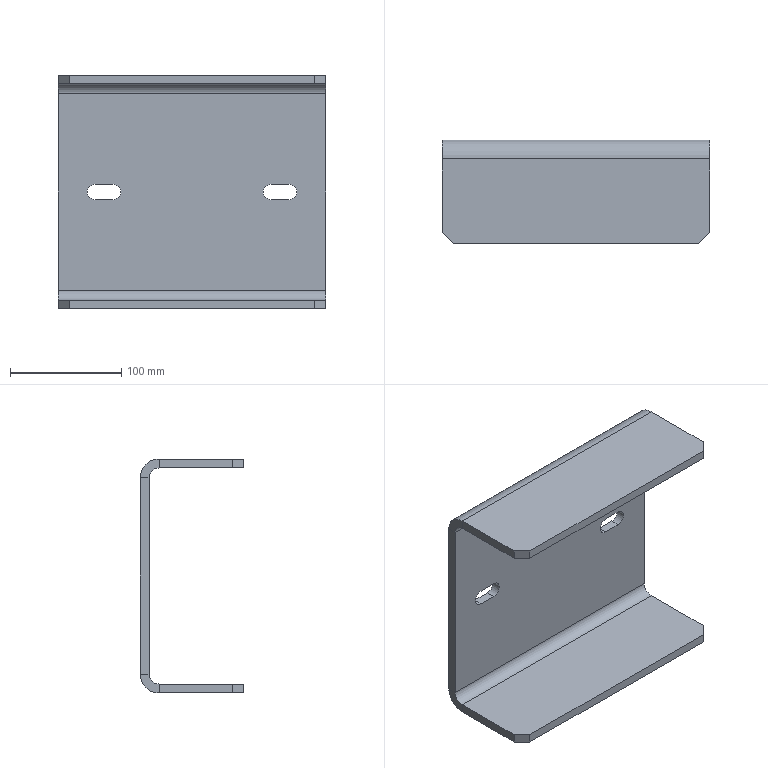Part | STEP file | _10001 | 1 solid | 34 faces | box 240 x 93 x 210 mm | volume 700527 mm3 | plane 26 | cylinder 8 | commonest cylinder face diameters 14 x4 18 x2 34 x2
STEP:
#1=CARTESIAN_POINT('',(71.,93.,235.5));
#2=VERTEX_POINT('',#1);
#3=CARTESIAN_POINT('',(71.,93.,221.5));
#4=VERTEX_POINT('',#3);
#5=CARTESIAN_POINT('',(71.,93.,228.5));
#6=DIRECTION('',(0.,-1.,0.));
#7=DIRECTION('',(0.,0.,1.));
#8=AXIS2_PLACEMENT_3D('',#5,#6,#7);
#9=CIRCLE('',#8,7.);
#10=EDGE_CURVE('',#2,#4,#9,.T.);
#11=ORIENTED_EDGE('',*,*,#10,.F.);
#12=CARTESIAN_POINT('',(71.,85.,235.5));
#13=VERTEX_POINT('',#12);
#14=CARTESIAN_POINT('',(71.,93.,235.5));
#15=DIRECTION('',(0.,-1.,0.));
#16=VECTOR('',#15,1000.);
#17=LINE('',#14,#16);
#18=EDGE_CURVE('',#2,#13,#17,.T.);
#19=ORIENTED_EDGE('',*,*,#18,.T.);
#20=CARTESIAN_POINT('',(71.,85.,221.5));
#21=VERTEX_POINT('',#20);
#22=CARTESIAN_POINT('',(71.,85.,228.5));
#23=DIRECTION('',(0.,1.,0.));
#24=DIRECTION('',(0.,0.,-1.));
#25=AXIS2_PLACEMENT_3D('',#22,#23,#24);
#26=CIRCLE('',#25,7.);
#27=EDGE_CURVE('',#21,#13,#26,.T.);
#28=ORIENTED_EDGE('',*,*,#27,.F.);
#29=CARTESIAN_POINT('',(71.,85.,221.5));
#30=DIRECTION('',(0.,1.,0.));
#31=VECTOR('',#30,1000.);
#32=LINE('',#29,#31);
#33=EDGE_CURVE('',#21,#4,#32,.T.);
#34=ORIENTED_EDGE('',*,*,#33,.T.);
#35=EDGE_LOOP('',(#11,#19,#28,#34));
#36=FACE_OUTER_BOUND('',#35,.T.);
#37=CARTESIAN_POINT('',(71.,83.,228.5));
#38=DIRECTION('',(0.,1.,0.));
#39=DIRECTION('',(0.,0.,1.));
#40=AXIS2_PLACEMENT_3D('',#37,#38,#39);
#41=CYLINDRICAL_SURFACE('',#40,7.);
#42=ADVANCED_FACE('',(#36),#41,.F.);
#43=CARTESIAN_POINT('',(87.,93.,235.5));
#44=VERTEX_POINT('',#43);
#45=CARTESIAN_POINT('',(87.,93.,235.5));
#46=DIRECTION('',(-1.,0.,0.));
#47=VECTOR('',#46,1000.);
#48=LINE('',#45,#47);
#49=EDGE_CURVE('',#44,#2,#48,.T.);
#50=ORIENTED_EDGE('',*,*,#49,.F.);
#51=CARTESIAN_POINT('',(87.,85.,235.5));
#52=VERTEX_POINT('',#51);
#53=CARTESIAN_POINT('',(87.,85.,235.5));
#54=DIRECTION('',(0.,1.,0.));
#55=VECTOR('',#54,1000.);
#56=LINE('',#53,#55);
#57=EDGE_CURVE('',#52,#44,#56,.T.);
#58=ORIENTED_EDGE('',*,*,#57,.F.);
#59=CARTESIAN_POINT('',(87.,85.,235.5));
#60=DIRECTION('',(-1.,0.,0.));
#61=VECTOR('',#60,1000.);
#62=LINE('',#59,#61);
#63=EDGE_CURVE('',#52,#13,#62,.T.);
#64=ORIENTED_EDGE('',*,*,#63,.T.);
#65=ORIENTED_EDGE('',*,*,#18,.F.);
#66=EDGE_LOOP('',(#50,#58,#64,#65));
#67=FACE_OUTER_BOUND('',#66,.T.);
#68=CARTESIAN_POINT('',(71.,83.,235.5));
#69=DIRECTION('',(0.,0.,1.));
#70=DIRECTION('',(1.,0.,0.));
#71=AXIS2_PLACEMENT_3D('',#68,#69,#70);
#72=PLANE('',#71);
#73=ADVANCED_FACE('',(#67),#72,.F.);
#74=CARTESIAN_POINT('',(87.,93.,221.5));
#75=VERTEX_POINT('',#74);
#76=CARTESIAN_POINT('',(87.,93.,228.5));
#77=DIRECTION('',(0.,-1.,0.));
#78=DIRECTION('',(0.,0.,-1.));
#79=AXIS2_PLACEMENT_3D('',#76,#77,#78);
#80=CIRCLE('',#79,7.);
#81=EDGE_CURVE('',#75,#44,#80,.T.);
#82=ORIENTED_EDGE('',*,*,#81,.F.);
#83=CARTESIAN_POINT('',(87.,85.,221.5));
#84=VERTEX_POINT('',#83);
#85=CARTESIAN_POINT('',(87.,93.,221.5));
#86=DIRECTION('',(0.,-1.,0.));
#87=VECTOR('',#86,1000.);
#88=LINE('',#85,#87);
#89=EDGE_CURVE('',#75,#84,#88,.T.);
#90=ORIENTED_EDGE('',*,*,#89,.T.);
#91=CARTESIAN_POINT('',(87.,85.,228.5));
#92=DIRECTION('',(0.,1.,0.));
#93=DIRECTION('',(0.,0.,1.));
#94=AXIS2_PLACEMENT_3D('',#91,#92,#93);
#95=CIRCLE('',#94,7.);
#96=EDGE_CURVE('',#52,#84,#95,.T.);
#97=ORIENTED_EDGE('',*,*,#96,.F.);
#98=ORIENTED_EDGE('',*,*,#57,.T.);
#99=EDGE_LOOP('',(#82,#90,#97,#98));
#100=FACE_OUTER_BOUND('',#99,.T.);
#101=CARTESIAN_POINT('',(87.,83.,228.5));
#102=DIRECTION('',(0.,1.,0.));
#103=DIRECTION('',(0.,0.,1.));
#104=AXIS2_PLACEMENT_3D('',#101,#102,#103);
#105=CYLINDRICAL_SURFACE('',#104,7.);
#106=ADVANCED_FACE('',(#100),#105,.F.);
#107=CARTESIAN_POINT('',(71.,93.,221.5));
#108=DIRECTION('',(1.,0.,0.));
#109=VECTOR('',#108,1000.);
#110=LINE('',#107,#109);
#111=EDGE_CURVE('',#4,#75,#110,.T.);
#112=ORIENTED_EDGE('',*,*,#111,.F.);
#113=ORIENTED_EDGE('',*,*,#33,.F.);
#114=CARTESIAN_POINT('',(71.,85.,221.5));
#115=DIRECTION('',(1.,0.,0.));
#116=VECTOR('',#115,1000.);
#117=LINE('',#114,#116);
#118=EDGE_CURVE('',#21,#84,#117,.T.);
#119=ORIENTED_EDGE('',*,*,#118,.T.);
#120=ORIENTED_EDGE('',*,*,#89,.F.);
#121=EDGE_LOOP('',(#112,#113,#119,#120));
#122=FACE_OUTER_BOUND('',#121,.T.);
#123=CARTESIAN_POINT('',(71.,83.,221.5));
#124=DIRECTION('',(0.,0.,-1.));
#125=DIRECTION('',(0.,-1.,0.));
#126=AXIS2_PLACEMENT_3D('',#123,#124,#125);
#127=PLANE('',#126);
#128=ADVANCED_FACE('',(#122),#127,.F.);
#129=CARTESIAN_POINT('',(-87.,93.,235.5));
#130=VERTEX_POINT('',#129);
#131=CARTESIAN_POINT('',(-87.,93.,221.5));
#132=VERTEX_POINT('',#131);
#133=CARTESIAN_POINT('',(-87.,93.,228.5));
#134=DIRECTION('',(0.,-1.,0.));
#135=DIRECTION('',(0.,0.,1.));
#136=AXIS2_PLACEMENT_3D('',#133,#134,#135);
#137=CIRCLE('',#136,7.);
#138=EDGE_CURVE('',#130,#132,#137,.T.);
#139=ORIENTED_EDGE('',*,*,#138,.F.);
#140=CARTESIAN_POINT('',(-87.,85.,235.5));
#141=VERTEX_POINT('',#140);
#142=CARTESIAN_POINT('',(-87.,93.,235.5));
#143=DIRECTION('',(0.,-1.,0.));
#144=VECTOR('',#143,1000.);
#145=LINE('',#142,#144);
#146=EDGE_CURVE('',#130,#141,#145,.T.);
#147=ORIENTED_EDGE('',*,*,#146,.T.);
#148=CARTESIAN_POINT('',(-87.,85.,221.5));
#149=VERTEX_POINT('',#148);
#150=CARTESIAN_POINT('',(-87.,85.,228.5));
#151=DIRECTION('',(0.,1.,0.));
#152=DIRECTION('',(0.,0.,-1.));
#153=AXIS2_PLACEMENT_3D('',#150,#151,#152);
#154=CIRCLE('',#153,7.);
#155=EDGE_CURVE('',#149,#141,#154,.T.);
#156=ORIENTED_EDGE('',*,*,#155,.F.);
#157=CARTESIAN_POINT('',(-87.,85.,221.5));
#158=DIRECTION('',(0.,1.,0.));
#159=VECTOR('',#158,1000.);
#160=LINE('',#157,#159);
#161=EDGE_CURVE('',#149,#132,#160,.T.);
#162=ORIENTED_EDGE('',*,*,#161,.T.);
#163=EDGE_LOOP('',(#139,#147,#156,#162));
#164=FACE_OUTER_BOUND('',#163,.T.);
#165=CARTESIAN_POINT('',(-87.,83.,228.5));
#166=DIRECTION('',(0.,1.,0.));
#167=DIRECTION('',(0.,0.,1.));
#168=AXIS2_PLACEMENT_3D('',#165,#166,#167);
#169=CYLINDRICAL_SURFACE('',#168,7.);
#170=ADVANCED_FACE('',(#164),#169,.F.);
#171=CARTESIAN_POINT('',(-71.,93.,235.5));
#172=VERTEX_POINT('',#171);
#173=CARTESIAN_POINT('',(-71.,93.,235.5));
#174=DIRECTION('',(-1.,0.,0.));
#175=VECTOR('',#174,1000.);
#176=LINE('',#173,#175);
#177=EDGE_CURVE('',#172,#130,#176,.T.);
#178=ORIENTED_EDGE('',*,*,#177,.F.);
#179=CARTESIAN_POINT('',(-71.,85.,235.5));
#180=VERTEX_POINT('',#179);
#181=CARTESIAN_POINT('',(-71.,85.,235.5));
#182=DIRECTION('',(0.,1.,0.));
#183=VECTOR('',#182,1000.);
#184=LINE('',#181,#183);
#185=EDGE_CURVE('',#180,#172,#184,.T.);
#186=ORIENTED_EDGE('',*,*,#185,.F.);
#187=CARTESIAN_POINT('',(-71.,85.,235.5));
#188=DIRECTION('',(-1.,0.,0.));
#189=VECTOR('',#188,1000.);
#190=LINE('',#187,#189);
#191=EDGE_CURVE('',#180,#141,#190,.T.);
#192=ORIENTED_EDGE('',*,*,#191,.T.);
#193=ORIENTED_EDGE('',*,*,#146,.F.);
#194=EDGE_LOOP('',(#178,#186,#192,#193));
#195=FACE_OUTER_BOUND('',#194,.T.);
#196=CARTESIAN_POINT('',(-87.,83.,235.5));
#197=DIRECTION('',(0.,0.,1.));
#198=DIRECTION('',(1.,0.,0.));
#199=AXIS2_PLACEMENT_3D('',#196,#197,#198);
#200=PLANE('',#199);
#201=ADVANCED_FACE('',(#195),#200,.F.);
#202=CARTESIAN_POINT('',(-71.,93.,221.5));
#203=VERTEX_POINT('',#202);
#204=CARTESIAN_POINT('',(-71.,93.,228.5));
#205=DIRECTION('',(0.,-1.,0.));
#206=DIRECTION('',(0.,0.,-1.));
#207=AXIS2_PLACEMENT_3D('',#204,#205,#206);
#208=CIRCLE('',#207,7.);
#209=EDGE_CURVE('',#203,#172,#208,.T.);
#210=ORIENTED_EDGE('',*,*,#209,.F.);
#211=CARTESIAN_POINT('',(-71.,85.,221.5));
#212=VERTEX_POINT('',#211);
#213=CARTESIAN_POINT('',(-71.,93.,221.5));
#214=DIRECTION('',(0.,-1.,0.));
#215=VECTOR('',#214,1000.);
#216=LINE('',#213,#215);
#217=EDGE_CURVE('',#203,#212,#216,.T.);
#218=ORIENTED_EDGE('',*,*,#217,.T.);
#219=CARTESIAN_POINT('',(-71.,85.,228.5));
#220=DIRECTION('',(0.,1.,0.));
#221=DIRECTION('',(0.,0.,1.));
#222=AXIS2_PLACEMENT_3D('',#219,#220,#221);
#223=CIRCLE('',#222,7.);
#224=EDGE_CURVE('',#180,#212,#223,.T.);
#225=ORIENTED_EDGE('',*,*,#224,.F.);
#226=ORIENTED_EDGE('',*,*,#185,.T.);
#227=EDGE_LOOP('',(#210,#218,#225,#226));
#228=FACE_OUTER_BOUND('',#227,.T.);
#229=CARTESIAN_POINT('',(-71.,83.,228.5));
#230=DIRECTION('',(0.,1.,0.));
#231=DIRECTION('',(0.,0.,1.));
#232=AXIS2_PLACEMENT_3D('',#229,#230,#231);
#233=CYLINDRICAL_SURFACE('',#232,7.);
#234=ADVANCED_FACE('',(#228),#233,.F.);
#235=CARTESIAN_POINT('',(-87.,93.,221.5));
#236=DIRECTION('',(1.,0.,0.));
#237=VECTOR('',#236,1000.);
#238=LINE('',#235,#237);
#239=EDGE_CURVE('',#132,#203,#238,.T.);
#240=ORIENTED_EDGE('',*,*,#239,.F.);
#241=ORIENTED_EDGE('',*,*,#161,.F.);
#242=CARTESIAN_POINT('',(-87.,85.,221.5));
#243=DIRECTION('',(1.,0.,0.));
#244=VECTOR('',#243,1000.);
#245=LINE('',#242,#244);
#246=EDGE_CURVE('',#149,#212,#245,.T.);
#247=ORIENTED_EDGE('',*,*,#246,.T.);
#248=ORIENTED_EDGE('',*,*,#217,.F.);
#249=EDGE_LOOP('',(#240,#241,#247,#248));
#250=FACE_OUTER_BOUND('',#249,.T.);
#251=CARTESIAN_POINT('',(-87.,83.,221.5));
#252=DIRECTION('',(0.,0.,-1.));
#253=DIRECTION('',(0.,-1.,0.));
#254=AXIS2_PLACEMENT_3D('',#251,#252,#253);
#255=PLANE('',#254);
#256=ADVANCED_FACE('',(#250),#255,.F.);
#257=CARTESIAN_POINT('',(-110.,0.,325.5));
#258=VERTEX_POINT('',#257);
#259=CARTESIAN_POINT('',(-110.,0.,333.5));
#260=VERTEX_POINT('',#259);
#261=CARTESIAN_POINT('',(-110.,0.,325.5));
#262=DIRECTION('',(0.,0.,1.));
#263=VECTOR('',#262,1000.);
#264=LINE('',#261,#263);
#265=EDGE_CURVE('',#258,#260,#264,.T.);
#266=ORIENTED_EDGE('',*,*,#265,.T.);
#267=CARTESIAN_POINT('',(-120.,10.,333.5));
#268=VERTEX_POINT('',#267);
#269=CARTESIAN_POINT('',(-120.,10.,333.5));
#270=DIRECTION('',(0.7071,-0.7071,0.));
#271=VECTOR('',#270,1000.);
#272=LINE('',#269,#271);
#273=EDGE_CURVE('',#268,#260,#272,.T.);
#274=ORIENTED_EDGE('',*,*,#273,.F.);
#275=CARTESIAN_POINT('',(-120.,10.,325.5));
#276=VERTEX_POINT('',#275);
#277=CARTESIAN_POINT('',(-120.,10.,333.5));
#278=DIRECTION('',(0.,0.,-1.));
#279=VECTOR('',#278,1000.);
#280=LINE('',#277,#279);
#281=EDGE_CURVE('',#268,#276,#280,.T.);
#282=ORIENTED_EDGE('',*,*,#281,.T.);
#283=CARTESIAN_POINT('',(-110.,0.,325.5));
#284=DIRECTION('',(-0.7071,0.7071,0.));
#285=VECTOR('',#284,1000.);
#286=LINE('',#283,#285);
#287=EDGE_CURVE('',#258,#276,#286,.T.);
#288=ORIENTED_EDGE('',*,*,#287,.F.);
#289=EDGE_LOOP('',(#266,#274,#282,#288));
#290=FACE_OUTER_BOUND('',#289,.T.);
#291=CARTESIAN_POINT('',(-120.,10.,316.5));
#292=DIRECTION('',(0.7071,0.7071,0.));
#293=DIRECTION('',(0.,0.,-1.));
#294=AXIS2_PLACEMENT_3D('',#291,#292,#293);
#295=PLANE('',#294);
#296=ADVANCED_FACE('',(#290),#295,.F.);
#297=CARTESIAN_POINT('',(120.,10.,325.5));
#298=VERTEX_POINT('',#297);
#299=CARTESIAN_POINT('',(120.,10.,333.5));
#300=VERTEX_POINT('',#299);
#301=CARTESIAN_POINT('',(120.,10.,325.5));
#302=DIRECTION('',(0.,0.,1.));
#303=VECTOR('',#302,1000.);
#304=LINE('',#301,#303);
#305=EDGE_CURVE('',#298,#300,#304,.T.);
#306=ORIENTED_EDGE('',*,*,#305,.T.);
#307=CARTESIAN_POINT('',(110.,0.,333.5));
#308=VERTEX_POINT('',#307);
#309=CARTESIAN_POINT('',(110.,0.,333.5));
#310=DIRECTION('',(0.7071,0.7071,0.));
#311=VECTOR('',#310,1000.);
#312=LINE('',#309,#311);
#313=EDGE_CURVE('',#308,#300,#312,.T.);
#314=ORIENTED_EDGE('',*,*,#313,.F.);
#315=CARTESIAN_POINT('',(110.,0.,325.5));
#316=VERTEX_POINT('',#315);
#317=CARTESIAN_POINT('',(110.,0.,333.5));
#318=DIRECTION('',(0.,0.,-1.));
#319=VECTOR('',#318,1000.);
#320=LINE('',#317,#319);
#321=EDGE_CURVE('',#308,#316,#320,.T.);
#322=ORIENTED_EDGE('',*,*,#321,.T.);
#323=CARTESIAN_POINT('',(120.,10.,325.5));
#324=DIRECTION('',(-0.7071,-0.7071,0.));
#325=VECTOR('',#324,1000.);
#326=LINE('',#323,#325);
#327=EDGE_CURVE('',#298,#316,#326,.T.);
#328=ORIENTED_EDGE('',*,*,#327,.F.);
#329=EDGE_LOOP('',(#306,#314,#322,#328));
#330=FACE_OUTER_BOUND('',#329,.T.);
#331=CARTESIAN_POINT('',(110.,0.,325.5));
#332=DIRECTION('',(-0.7071,0.7071,0.));
#333=DIRECTION('',(0.,0.,1.));
#334=AXIS2_PLACEMENT_3D('',#331,#332,#333);
#335=PLANE('',#334);
#336=ADVANCED_FACE('',(#330),#335,.F.);
#337=ORIENTED_EDGE('',*,*,#305,.F.);
#338=CARTESIAN_POINT('',(120.,76.,325.5));
#339=VERTEX_POINT('',#338);
#340=CARTESIAN_POINT('',(120.,76.,325.5));
#341=DIRECTION('',(0.,-1.,0.));
#342=VECTOR('',#341,1000.);
#343=LINE('',#340,#342);
#344=EDGE_CURVE('',#339,#298,#343,.T.);
#345=ORIENTED_EDGE('',*,*,#344,.F.);
#346=CARTESIAN_POINT('',(120.,76.,333.5));
#347=VERTEX_POINT('',#346);
#348=CARTESIAN_POINT('',(120.,76.,333.5));
#349=DIRECTION('',(0.,0.,-1.));
#350=VECTOR('',#349,1000.);
#351=LINE('',#348,#350);
#352=EDGE_CURVE('',#347,#339,#351,.T.);
#353=ORIENTED_EDGE('',*,*,#352,.F.);
#354=CARTESIAN_POINT('',(120.,76.,333.5));
#355=DIRECTION('',(0.,-1.,0.));
#356=VECTOR('',#355,1000.);
#357=LINE('',#354,#356);
#358=EDGE_CURVE('',#347,#300,#357,.T.);
#359=ORIENTED_EDGE('',*,*,#358,.T.);
#360=EDGE_LOOP('',(#337,#345,#353,#359));
#361=FACE_OUTER_BOUND('',#360,.T.);
#362=CARTESIAN_POINT('',(120.,76.,140.5));
#363=DIRECTION('',(1.,0.,0.));
#364=DIRECTION('',(0.,1.,0.));
#365=AXIS2_PLACEMENT_3D('',#362,#363,#364);
#366=PLANE('',#365);
#367=ADVANCED_FACE('',(#361),#366,.T.);
#368=CARTESIAN_POINT('',(120.,93.,316.5));
#369=VERTEX_POINT('',#368);
#370=CARTESIAN_POINT('',(120.,76.,316.5));
#371=DIRECTION('',(1.,0.,0.));
#372=DIRECTION('',(0.,1.,0.));
#373=AXIS2_PLACEMENT_3D('',#370,#371,#372);
#374=CIRCLE('',#373,17.);
#375=EDGE_CURVE('',#369,#347,#374,.T.);
#376=ORIENTED_EDGE('',*,*,#375,.T.);
#377=ORIENTED_EDGE('',*,*,#352,.T.);
#378=CARTESIAN_POINT('',(120.,85.,316.5));
#379=VERTEX_POINT('',#378);
#380=CARTESIAN_POINT('',(120.,76.,316.5));
#381=DIRECTION('',(-1.,0.,0.));
#382=DIRECTION('',(0.,0.,1.));
#383=AXIS2_PLACEMENT_3D('',#380,#381,#382);
#384=CIRCLE('',#383,9.);
#385=EDGE_CURVE('',#339,#379,#384,.T.);
#386=ORIENTED_EDGE('',*,*,#385,.T.);
#387=CARTESIAN_POINT('',(120.,85.,316.5));
#388=DIRECTION('',(0.,1.,0.));
#389=VECTOR('',#388,1000.);
#390=LINE('',#387,#389);
#391=EDGE_CURVE('',#379,#369,#390,.T.);
#392=ORIENTED_EDGE('',*,*,#391,.T.);
#393=EDGE_LOOP('',(#376,#377,#386,#392));
#394=FACE_OUTER_BOUND('',#393,.T.);
#395=CARTESIAN_POINT('',(120.,93.,316.5));
#396=DIRECTION('',(1.,0.,0.));
#397=DIRECTION('',(0.,1.,0.));
#398=AXIS2_PLACEMENT_3D('',#395,#396,#397);
#399=PLANE('',#398);
#400=ADVANCED_FACE('',(#394),#399,.T.);
#401=CARTESIAN_POINT('',(-120.,76.,333.5));
#402=VERTEX_POINT('',#401);
#403=CARTESIAN_POINT('',(-120.,76.,333.5));
#404=DIRECTION('',(1.,0.,0.));
#405=VECTOR('',#404,1000.);
#406=LINE('',#403,#405);
#407=EDGE_CURVE('',#402,#347,#406,.T.);
#408=ORIENTED_EDGE('',*,*,#407,.T.);
#409=ORIENTED_EDGE('',*,*,#375,.F.);
#410=CARTESIAN_POINT('',(-120.,93.,316.5));
#411=VERTEX_POINT('',#410);
#412=CARTESIAN_POINT('',(120.,93.,316.5));
#413=DIRECTION('',(-1.,0.,0.));
#414=VECTOR('',#413,1000.);
#415=LINE('',#412,#414);
#416=EDGE_CURVE('',#369,#411,#415,.T.);
#417=ORIENTED_EDGE('',*,*,#416,.T.);
#418=CARTESIAN_POINT('',(-120.,76.,316.5));
#419=DIRECTION('',(-1.,0.,0.));
#420=DIRECTION('',(0.,0.,1.));
#421=AXIS2_PLACEMENT_3D('',#418,#419,#420);
#422=CIRCLE('',#421,17.);
#423=EDGE_CURVE('',#402,#411,#422,.T.);
#424=ORIENTED_EDGE('',*,*,#423,.F.);
#425=EDGE_LOOP('',(#408,#409,#417,#424));
#426=FACE_OUTER_BOUND('',#425,.T.);
#427=CARTESIAN_POINT('',(120.,76.,316.5));
#428=DIRECTION('',(-1.,0.,0.));
#429=DIRECTION('',(0.,0.,1.));
#430=AXIS2_PLACEMENT_3D('',#427,#428,#429);
#431=CYLINDRICAL_SURFACE('',#430,17.);
#432=ADVANCED_FACE('',(#426),#431,.T.);
#433=ORIENTED_EDGE('',*,*,#273,.T.);
#434=CARTESIAN_POINT('',(-110.,0.,333.5));
#435=DIRECTION('',(1.,0.,0.));
#436=VECTOR('',#435,1000.);
#437=LINE('',#434,#436);
#438=EDGE_CURVE('',#260,#308,#437,.T.);
#439=ORIENTED_EDGE('',*,*,#438,.T.);
#440=ORIENTED_EDGE('',*,*,#313,.T.);
#441=ORIENTED_EDGE('',*,*,#358,.F.);
#442=ORIENTED_EDGE('',*,*,#407,.F.);
#443=CARTESIAN_POINT('',(-120.,76.,333.5));
#444=DIRECTION('',(0.,-1.,0.));
#445=VECTOR('',#444,1000.);
#446=LINE('',#443,#445);
#447=EDGE_CURVE('',#402,#268,#446,.T.);
#448=ORIENTED_EDGE('',*,*,#447,.T.);
#449=EDGE_LOOP('',(#433,#439,#440,#441,#442,#448));
#450=FACE_OUTER_BOUND('',#449,.T.);
#451=CARTESIAN_POINT('',(120.,0.,333.5));
#452=DIRECTION('',(0.,0.,1.));
#453=DIRECTION('',(1.,0.,0.));
#454=AXIS2_PLACEMENT_3D('',#451,#452,#453);
#455=PLANE('',#454);
#456=ADVANCED_FACE('',(#450),#455,.T.);
#457=ORIENTED_EDGE('',*,*,#265,.F.);
#458=CARTESIAN_POINT('',(-110.,0.,325.5));
#459=DIRECTION('',(1.,0.,0.));
#460=VECTOR('',#459,1000.);
#461=LINE('',#458,#460);
#462=EDGE_CURVE('',#258,#316,#461,.T.);
#463=ORIENTED_EDGE('',*,*,#462,.T.);
#464=ORIENTED_EDGE('',*,*,#321,.F.);
#465=ORIENTED_EDGE('',*,*,#438,.F.);
#466=EDGE_LOOP('',(#457,#463,#464,#465));
#467=FACE_OUTER_BOUND('',#466,.T.);
#468=CARTESIAN_POINT('',(120.,0.,325.5));
#469=DIRECTION('',(0.,-1.,0.));
#470=DIRECTION('',(0.,0.,-1.));
#471=AXIS2_PLACEMENT_3D('',#468,#469,#470);
#472=PLANE('',#471);
#473=ADVANCED_FACE('',(#467),#472,.T.);
#474=ORIENTED_EDGE('',*,*,#287,.T.);
#475=CARTESIAN_POINT('',(-120.,76.,325.5));
#476=VERTEX_POINT('',#475);
#477=CARTESIAN_POINT('',(-120.,76.,325.5));
#478=DIRECTION('',(0.,-1.,0.));
#479=VECTOR('',#478,1000.);
#480=LINE('',#477,#479);
#481=EDGE_CURVE('',#476,#276,#480,.T.);
#482=ORIENTED_EDGE('',*,*,#481,.F.);
#483=CARTESIAN_POINT('',(120.,76.,325.5));
#484=DIRECTION('',(-1.,0.,0.));
#485=VECTOR('',#484,1000.);
#486=LINE('',#483,#485);
#487=EDGE_CURVE('',#339,#476,#486,.T.);
#488=ORIENTED_EDGE('',*,*,#487,.F.);
#489=ORIENTED_EDGE('',*,*,#344,.T.);
#490=ORIENTED_EDGE('',*,*,#327,.T.);
#491=ORIENTED_EDGE('',*,*,#462,.F.);
#492=EDGE_LOOP('',(#474,#482,#488,#489,#490,#491));
#493=FACE_OUTER_BOUND('',#492,.T.);
#494=CARTESIAN_POINT('',(120.,0.,325.5));
#495=DIRECTION('',(0.,0.,1.));
#496=DIRECTION('',(1.,0.,0.));
#497=AXIS2_PLACEMENT_3D('',#494,#495,#496);
#498=PLANE('',#497);
#499=ADVANCED_FACE('',(#493),#498,.F.);
#500=ORIENTED_EDGE('',*,*,#281,.F.);
#501=ORIENTED_EDGE('',*,*,#447,.F.);
#502=CARTESIAN_POINT('',(-120.,76.,325.5));
#503=DIRECTION('',(0.,0.,1.));
#504=VECTOR('',#503,1000.);
#505=LINE('',#502,#504);
#506=EDGE_CURVE('',#476,#402,#505,.T.);
#507=ORIENTED_EDGE('',*,*,#506,.F.);
#508=ORIENTED_EDGE('',*,*,#481,.T.);
#509=EDGE_LOOP('',(#500,#501,#507,#508));
#510=FACE_OUTER_BOUND('',#509,.T.);
#511=CARTESIAN_POINT('',(-120.,85.,316.5));
#512=DIRECTION('',(-1.,0.,0.));
#513=DIRECTION('',(0.,0.,1.));
#514=AXIS2_PLACEMENT_3D('',#511,#512,#513);
#515=PLANE('',#514);
#516=ADVANCED_FACE('',(#510),#515,.T.);
#517=ORIENTED_EDGE('',*,*,#423,.T.);
#518=CARTESIAN_POINT('',(-120.,85.,316.5));
#519=VERTEX_POINT('',#518);
#520=CARTESIAN_POINT('',(-120.,93.,316.5));
#521=DIRECTION('',(0.,-1.,0.));
#522=VECTOR('',#521,1000.);
#523=LINE('',#520,#522);
#524=EDGE_CURVE('',#411,#519,#523,.T.);
#525=ORIENTED_EDGE('',*,*,#524,.T.);
#526=CARTESIAN_POINT('',(-120.,76.,316.5));
#527=DIRECTION('',(1.,0.,0.));
#528=DIRECTION('',(0.,1.,0.));
#529=AXIS2_PLACEMENT_3D('',#526,#527,#528);
#530=CIRCLE('',#529,9.);
#531=EDGE_CURVE('',#519,#476,#530,.T.);
#532=ORIENTED_EDGE('',*,*,#531,.T.);
#533=ORIENTED_EDGE('',*,*,#506,.T.);
#534=EDGE_LOOP('',(#517,#525,#532,#533));
#535=FACE_OUTER_BOUND('',#534,.T.);
#536=CARTESIAN_POINT('',(-120.,76.,333.5));
#537=DIRECTION('',(-1.,0.,0.));
#538=DIRECTION('',(0.,0.,1.));
#539=AXIS2_PLACEMENT_3D('',#536,#537,#538);
#540=PLANE('',#539);
#541=ADVANCED_FACE('',(#535),#540,.T.);
#542=CARTESIAN_POINT('',(-120.,85.,316.5));
#543=DIRECTION('',(1.,0.,0.));
#544=VECTOR('',#543,1000.);
#545=LINE('',#542,#544);
#546=EDGE_CURVE('',#519,#379,#545,.T.);
#547=ORIENTED_EDGE('',*,*,#546,.T.);
#548=ORIENTED_EDGE('',*,*,#385,.F.);
#549=ORIENTED_EDGE('',*,*,#487,.T.);
#550=ORIENTED_EDGE('',*,*,#531,.F.);
#551=EDGE_LOOP('',(#547,#548,#549,#550));
#552=FACE_OUTER_BOUND('',#551,.T.);
#553=CARTESIAN_POINT('',(120.,76.,316.5));
#554=DIRECTION('',(-1.,0.,0.));
#555=DIRECTION('',(0.,0.,1.));
#556=AXIS2_PLACEMENT_3D('',#553,#554,#555);
#557=CYLINDRICAL_SURFACE('',#556,9.);
#558=ADVANCED_FACE('',(#552),#557,.F.);
#559=ORIENTED_EDGE('',*,*,#27,.T.);
#560=ORIENTED_EDGE('',*,*,#63,.F.);
#561=ORIENTED_EDGE('',*,*,#96,.T.);
#562=ORIENTED_EDGE('',*,*,#118,.F.);
#563=EDGE_LOOP('',(#559,#560,#561,#562));
#564=FACE_BOUND('',#563,.T.);
#565=ORIENTED_EDGE('',*,*,#155,.T.);
#566=ORIENTED_EDGE('',*,*,#191,.F.);
#567=ORIENTED_EDGE('',*,*,#224,.T.);
#568=ORIENTED_EDGE('',*,*,#246,.F.);
#569=EDGE_LOOP('',(#565,#566,#567,#568));
#570=FACE_BOUND('',#569,.T.);
#571=CARTESIAN_POINT('',(120.,85.,140.5));
#572=VERTEX_POINT('',#571);
#573=CARTESIAN_POINT('',(-120.,85.,140.5));
#574=VERTEX_POINT('',#573);
#575=CARTESIAN_POINT('',(120.,85.,140.5));
#576=DIRECTION('',(-1.,0.,0.));
#577=VECTOR('',#576,1000.);
#578=LINE('',#575,#577);
#579=EDGE_CURVE('',#572,#574,#578,.T.);
#580=ORIENTED_EDGE('',*,*,#579,.F.);
#581=CARTESIAN_POINT('',(120.,85.,140.5));
#582=DIRECTION('',(0.,0.,1.));
#583=VECTOR('',#582,1000.);
#584=LINE('',#581,#583);
#585=EDGE_CURVE('',#572,#379,#584,.T.);
#586=ORIENTED_EDGE('',*,*,#585,.T.);
#587=ORIENTED_EDGE('',*,*,#546,.F.);
#588=CARTESIAN_POINT('',(-120.,85.,140.5));
#589=DIRECTION('',(0.,0.,1.));
#590=VECTOR('',#589,1000.);
#591=LINE('',#588,#590);
#592=EDGE_CURVE('',#574,#519,#591,.T.);
#593=ORIENTED_EDGE('',*,*,#592,.F.);
#594=EDGE_LOOP('',(#580,#586,#587,#593));
#595=FACE_OUTER_BOUND('',#594,.T.);
#596=CARTESIAN_POINT('',(120.,85.,333.5));
#597=DIRECTION('',(0.,1.,0.));
#598=DIRECTION('',(1.,0.,0.));
#599=AXIS2_PLACEMENT_3D('',#596,#597,#598);
#600=PLANE('',#599);
#601=ADVANCED_FACE('',(#564,#570,#595),#600,.F.);
#602=CARTESIAN_POINT('',(-120.,76.,131.5));
#603=VERTEX_POINT('',#602);
#604=CARTESIAN_POINT('',(120.,76.,131.5));
#605=VERTEX_POINT('',#604);
#606=CARTESIAN_POINT('',(-120.,76.,131.5));
#607=DIRECTION('',(1.,0.,0.));
#608=VECTOR('',#607,1000.);
#609=LINE('',#606,#608);
#610=EDGE_CURVE('',#603,#605,#609,.T.);
#611=ORIENTED_EDGE('',*,*,#610,.T.);
#612=CARTESIAN_POINT('',(120.,76.,140.5));
#613=DIRECTION('',(-1.,0.,0.));
#614=DIRECTION('',(0.,1.,0.));
#615=AXIS2_PLACEMENT_3D('',#612,#613,#614);
#616=CIRCLE('',#615,9.);
#617=EDGE_CURVE('',#572,#605,#616,.T.);
#618=ORIENTED_EDGE('',*,*,#617,.F.);
#619=ORIENTED_EDGE('',*,*,#579,.T.);
#620=CARTESIAN_POINT('',(-120.,76.,140.5));
#621=DIRECTION('',(1.,0.,0.));
#622=DIRECTION('',(0.,0.,-1.));
#623=AXIS2_PLACEMENT_3D('',#620,#621,#622);
#624=CIRCLE('',#623,9.);
#625=EDGE_CURVE('',#603,#574,#624,.T.);
#626=ORIENTED_EDGE('',*,*,#625,.F.);
#627=EDGE_LOOP('',(#611,#618,#619,#626));
#628=FACE_OUTER_BOUND('',#627,.T.);
#629=CARTESIAN_POINT('',(120.,76.,140.5));
#630=DIRECTION('',(-1.,0.,0.));
#631=DIRECTION('',(0.,0.,1.));
#632=AXIS2_PLACEMENT_3D('',#629,#630,#631);
#633=CYLINDRICAL_SURFACE('',#632,9.);
#634=ADVANCED_FACE('',(#628),#633,.F.);
#635=CARTESIAN_POINT('',(-110.,0.,123.5));
#636=VERTEX_POINT('',#635);
#637=CARTESIAN_POINT('',(-110.,0.,131.5));
#638=VERTEX_POINT('',#637);
#639=CARTESIAN_POINT('',(-110.,0.,123.5));
#640=DIRECTION('',(0.,0.,1.));
#641=VECTOR('',#640,1000.);
#642=LINE('',#639,#641);
#643=EDGE_CURVE('',#636,#638,#642,.T.);
#644=ORIENTED_EDGE('',*,*,#643,.T.);
#645=CARTESIAN_POINT('',(-120.,10.,131.5));
#646=VERTEX_POINT('',#645);
#647=CARTESIAN_POINT('',(-120.,10.,131.5));
#648=DIRECTION('',(0.7071,-0.7071,0.));
#649=VECTOR('',#648,1000.);
#650=LINE('',#647,#649);
#651=EDGE_CURVE('',#646,#638,#650,.T.);
#652=ORIENTED_EDGE('',*,*,#651,.F.);
#653=CARTESIAN_POINT('',(-120.,10.,123.5));
#654=VERTEX_POINT('',#653);
#655=CARTESIAN_POINT('',(-120.,10.,131.5));
#656=DIRECTION('',(0.,0.,-1.));
#657=VECTOR('',#656,1000.);
#658=LINE('',#655,#657);
#659=EDGE_CURVE('',#646,#654,#658,.T.);
#660=ORIENTED_EDGE('',*,*,#659,.T.);
#661=CARTESIAN_POINT('',(-110.,0.,123.5));
#662=DIRECTION('',(-0.7071,0.7071,0.));
#663=VECTOR('',#662,1000.);
#664=LINE('',#661,#663);
#665=EDGE_CURVE('',#636,#654,#664,.T.);
#666=ORIENTED_EDGE('',*,*,#665,.F.);
#667=EDGE_LOOP('',(#644,#652,#660,#666));
#668=FACE_OUTER_BOUND('',#667,.T.);
#669=CARTESIAN_POINT('',(-120.,10.,140.5));
#670=DIRECTION('',(-0.7071,-0.7071,0.));
#671=DIRECTION('',(-0.7071,0.7071,0.));
#672=AXIS2_PLACEMENT_3D('',#669,#670,#671);
#673=PLANE('',#672);
#674=ADVANCED_FACE('',(#668),#673,.T.);
#675=CARTESIAN_POINT('',(120.,10.,123.5));
#676=VERTEX_POINT('',#675);
#677=CARTESIAN_POINT('',(120.,10.,131.5));
#678=VERTEX_POINT('',#677);
#679=CARTESIAN_POINT('',(120.,10.,123.5));
#680=DIRECTION('',(0.,0.,1.));
#681=VECTOR('',#680,1000.);
#682=LINE('',#679,#681);
#683=EDGE_CURVE('',#676,#678,#682,.T.);
#684=ORIENTED_EDGE('',*,*,#683,.T.);
#685=CARTESIAN_POINT('',(110.,0.,131.5));
#686=VERTEX_POINT('',#685);
#687=CARTESIAN_POINT('',(110.,0.,131.5));
#688=DIRECTION('',(0.7071,0.7071,0.));
#689=VECTOR('',#688,1000.);
#690=LINE('',#687,#689);
#691=EDGE_CURVE('',#686,#678,#690,.T.);
#692=ORIENTED_EDGE('',*,*,#691,.F.);
#693=CARTESIAN_POINT('',(110.,0.,123.5));
#694=VERTEX_POINT('',#693);
#695=CARTESIAN_POINT('',(110.,0.,131.5));
#696=DIRECTION('',(0.,0.,-1.));
#697=VECTOR('',#696,1000.);
#698=LINE('',#695,#697);
#699=EDGE_CURVE('',#686,#694,#698,.T.);
#700=ORIENTED_EDGE('',*,*,#699,.T.);
#701=CARTESIAN_POINT('',(120.,10.,123.5));
#702=DIRECTION('',(-0.7071,-0.7071,0.));
#703=VECTOR('',#702,1000.);
#704=LINE('',#701,#703);
#705=EDGE_CURVE('',#676,#694,#704,.T.);
#706=ORIENTED_EDGE('',*,*,#705,.F.);
#707=EDGE_LOOP('',(#684,#692,#700,#706));
#708=FACE_OUTER_BOUND('',#707,.T.);
#709=CARTESIAN_POINT('',(110.,0.,123.5));
#710=DIRECTION('',(-0.7071,0.7071,0.));
#711=DIRECTION('',(0.,0.,1.));
#712=AXIS2_PLACEMENT_3D('',#709,#710,#711);
#713=PLANE('',#712);
#714=ADVANCED_FACE('',(#708),#713,.F.);
#715=ORIENTED_EDGE('',*,*,#643,.F.);
#716=CARTESIAN_POINT('',(-110.,0.,123.5));
#717=DIRECTION('',(1.,0.,0.));
#718=VECTOR('',#717,1000.);
#719=LINE('',#716,#718);
#720=EDGE_CURVE('',#636,#694,#719,.T.);
#721=ORIENTED_EDGE('',*,*,#720,.T.);
#722=ORIENTED_EDGE('',*,*,#699,.F.);
#723=CARTESIAN_POINT('',(-110.,0.,131.5));
#724=DIRECTION('',(1.,0.,0.));
#725=VECTOR('',#724,1000.);
#726=LINE('',#723,#725);
#727=EDGE_CURVE('',#638,#686,#726,.T.);
#728=ORIENTED_EDGE('',*,*,#727,.F.);
#729=EDGE_LOOP('',(#715,#721,#722,#728));
#730=FACE_OUTER_BOUND('',#729,.T.);
#731=CARTESIAN_POINT('',(120.,0.,123.5));
#732=DIRECTION('',(0.,-1.,0.));
#733=DIRECTION('',(0.,0.,-1.));
#734=AXIS2_PLACEMENT_3D('',#731,#732,#733);
#735=PLANE('',#734);
#736=ADVANCED_FACE('',(#730),#735,.T.);
#737=ORIENTED_EDGE('',*,*,#665,.T.);
#738=CARTESIAN_POINT('',(-120.,76.,123.5));
#739=VERTEX_POINT('',#738);
#740=CARTESIAN_POINT('',(-120.,10.,123.5));
#741=DIRECTION('',(0.,1.,0.));
#742=VECTOR('',#741,1000.);
#743=LINE('',#740,#742);
#744=EDGE_CURVE('',#654,#739,#743,.T.);
#745=ORIENTED_EDGE('',*,*,#744,.T.);
#746=CARTESIAN_POINT('',(120.,76.,123.5));
#747=VERTEX_POINT('',#746);
#748=CARTESIAN_POINT('',(120.,76.,123.5));
#749=DIRECTION('',(-1.,0.,0.));
#750=VECTOR('',#749,1000.);
#751=LINE('',#748,#750);
#752=EDGE_CURVE('',#747,#739,#751,.T.);
#753=ORIENTED_EDGE('',*,*,#752,.F.);
#754=CARTESIAN_POINT('',(120.,10.,123.5));
#755=DIRECTION('',(0.,1.,0.));
#756=VECTOR('',#755,1000.);
#757=LINE('',#754,#756);
#758=EDGE_CURVE('',#676,#747,#757,.T.);
#759=ORIENTED_EDGE('',*,*,#758,.F.);
#760=ORIENTED_EDGE('',*,*,#705,.T.);
#761=ORIENTED_EDGE('',*,*,#720,.F.);
#762=EDGE_LOOP('',(#737,#745,#753,#759,#760,#761));
#763=FACE_OUTER_BOUND('',#762,.T.);
#764=CARTESIAN_POINT('',(120.,93.,123.5));
#765=DIRECTION('',(0.,0.,-1.));
#766=DIRECTION('',(0.,-1.,0.));
#767=AXIS2_PLACEMENT_3D('',#764,#765,#766);
#768=PLANE('',#767);
#769=ADVANCED_FACE('',(#763),#768,.T.);
#770=ORIENTED_EDGE('',*,*,#659,.F.);
#771=CARTESIAN_POINT('',(-120.,10.,131.5));
#772=DIRECTION('',(0.,1.,0.));
#773=VECTOR('',#772,1000.);
#774=LINE('',#771,#773);
#775=EDGE_CURVE('',#646,#603,#774,.T.);
#776=ORIENTED_EDGE('',*,*,#775,.T.);
#777=CARTESIAN_POINT('',(-120.,76.,123.5));
#778=DIRECTION('',(0.,0.,1.));
#779=VECTOR('',#778,1000.);
#780=LINE('',#777,#779);
#781=EDGE_CURVE('',#739,#603,#780,.T.);
#782=ORIENTED_EDGE('',*,*,#781,.F.);
#783=ORIENTED_EDGE('',*,*,#744,.F.);
#784=EDGE_LOOP('',(#770,#776,#782,#783));
#785=FACE_OUTER_BOUND('',#784,.T.);
#786=CARTESIAN_POINT('',(-120.,76.,140.5));
#787=DIRECTION('',(1.,0.,0.));
#788=DIRECTION('',(0.,1.,0.));
#789=AXIS2_PLACEMENT_3D('',#786,#787,#788);
#790=PLANE('',#789);
#791=ADVANCED_FACE('',(#785),#790,.F.);
#792=ORIENTED_EDGE('',*,*,#651,.T.);
#793=ORIENTED_EDGE('',*,*,#727,.T.);
#794=ORIENTED_EDGE('',*,*,#691,.T.);
#795=CARTESIAN_POINT('',(120.,10.,131.5));
#796=DIRECTION('',(0.,1.,0.));
#797=VECTOR('',#796,1000.);
#798=LINE('',#795,#797);
#799=EDGE_CURVE('',#678,#605,#798,.T.);
#800=ORIENTED_EDGE('',*,*,#799,.T.);
#801=ORIENTED_EDGE('',*,*,#610,.F.);
#802=ORIENTED_EDGE('',*,*,#775,.F.);
#803=EDGE_LOOP('',(#792,#793,#794,#800,#801,#802));
#804=FACE_OUTER_BOUND('',#803,.T.);
#805=CARTESIAN_POINT('',(120.,93.,131.5));
#806=DIRECTION('',(0.,0.,-1.));
#807=DIRECTION('',(0.,-1.,0.));
#808=AXIS2_PLACEMENT_3D('',#805,#806,#807);
#809=PLANE('',#808);
#810=ADVANCED_FACE('',(#804),#809,.F.);
#811=ORIENTED_EDGE('',*,*,#683,.F.);
#812=ORIENTED_EDGE('',*,*,#758,.T.);
#813=CARTESIAN_POINT('',(120.,76.,131.5));
#814=DIRECTION('',(0.,0.,-1.));
#815=VECTOR('',#814,1000.);
#816=LINE('',#813,#815);
#817=EDGE_CURVE('',#605,#747,#816,.T.);
#818=ORIENTED_EDGE('',*,*,#817,.F.);
#819=ORIENTED_EDGE('',*,*,#799,.F.);
#820=EDGE_LOOP('',(#811,#812,#818,#819));
#821=FACE_OUTER_BOUND('',#820,.T.);
#822=CARTESIAN_POINT('',(120.,85.,140.5));
#823=DIRECTION('',(1.,0.,0.));
#824=DIRECTION('',(0.,1.,0.));
#825=AXIS2_PLACEMENT_3D('',#822,#823,#824);
#826=PLANE('',#825);
#827=ADVANCED_FACE('',(#821),#826,.T.);
#828=CARTESIAN_POINT('',(120.,93.,140.5));
#829=VERTEX_POINT('',#828);
#830=CARTESIAN_POINT('',(120.,76.,140.5));
#831=DIRECTION('',(1.,0.,0.));
#832=DIRECTION('',(0.,0.,-1.));
#833=AXIS2_PLACEMENT_3D('',#830,#831,#832);
#834=CIRCLE('',#833,17.);
#835=EDGE_CURVE('',#747,#829,#834,.T.);
#836=ORIENTED_EDGE('',*,*,#835,.T.);
#837=CARTESIAN_POINT('',(120.,93.,140.5));
#838=DIRECTION('',(0.,-1.,0.));
#839=VECTOR('',#838,1000.);
#840=LINE('',#837,#839);
#841=EDGE_CURVE('',#829,#572,#840,.T.);
#842=ORIENTED_EDGE('',*,*,#841,.T.);
#843=ORIENTED_EDGE('',*,*,#617,.T.);
#844=ORIENTED_EDGE('',*,*,#817,.T.);
#845=EDGE_LOOP('',(#836,#842,#843,#844));
#846=FACE_OUTER_BOUND('',#845,.T.);
#847=CARTESIAN_POINT('',(120.,76.,123.5));
#848=DIRECTION('',(1.,0.,0.));
#849=DIRECTION('',(0.,1.,0.));
#850=AXIS2_PLACEMENT_3D('',#847,#848,#849);
#851=PLANE('',#850);
#852=ADVANCED_FACE('',(#846),#851,.T.);
#853=ORIENTED_EDGE('',*,*,#391,.F.);
#854=ORIENTED_EDGE('',*,*,#585,.F.);
#855=ORIENTED_EDGE('',*,*,#841,.F.);
#856=CARTESIAN_POINT('',(120.,93.,140.5));
#857=DIRECTION('',(0.,0.,1.));
#858=VECTOR('',#857,1000.);
#859=LINE('',#856,#858);
#860=EDGE_CURVE('',#829,#369,#859,.T.);
#861=ORIENTED_EDGE('',*,*,#860,.T.);
#862=EDGE_LOOP('',(#853,#854,#855,#861));
#863=FACE_OUTER_BOUND('',#862,.T.);
#864=CARTESIAN_POINT('',(120.,76.,325.5));
#865=DIRECTION('',(1.,0.,0.));
#866=DIRECTION('',(0.,1.,0.));
#867=AXIS2_PLACEMENT_3D('',#864,#865,#866);
#868=PLANE('',#867);
#869=ADVANCED_FACE('',(#863),#868,.T.);
#870=ORIENTED_EDGE('',*,*,#111,.T.);
#871=ORIENTED_EDGE('',*,*,#81,.T.);
#872=ORIENTED_EDGE('',*,*,#49,.T.);
#873=ORIENTED_EDGE('',*,*,#10,.T.);
#874=EDGE_LOOP('',(#870,#871,#872,#873));
#875=FACE_BOUND('',#874,.T.);
#876=ORIENTED_EDGE('',*,*,#239,.T.);
#877=ORIENTED_EDGE('',*,*,#209,.T.);
#878=ORIENTED_EDGE('',*,*,#177,.T.);
#879=ORIENTED_EDGE('',*,*,#138,.T.);
#880=EDGE_LOOP('',(#876,#877,#878,#879));
#881=FACE_BOUND('',#880,.T.);
#882=ORIENTED_EDGE('',*,*,#416,.F.);
#883=ORIENTED_EDGE('',*,*,#860,.F.);
#884=CARTESIAN_POINT('',(-120.,93.,140.5));
#885=VERTEX_POINT('',#884);
#886=CARTESIAN_POINT('',(-120.,93.,140.5));
#887=DIRECTION('',(1.,0.,0.));
#888=VECTOR('',#887,1000.);
#889=LINE('',#886,#888);
#890=EDGE_CURVE('',#885,#829,#889,.T.);
#891=ORIENTED_EDGE('',*,*,#890,.F.);
#892=CARTESIAN_POINT('',(-120.,93.,140.5));
#893=DIRECTION('',(0.,0.,1.));
#894=VECTOR('',#893,1000.);
#895=LINE('',#892,#894);
#896=EDGE_CURVE('',#885,#411,#895,.T.);
#897=ORIENTED_EDGE('',*,*,#896,.T.);
#898=EDGE_LOOP('',(#882,#883,#891,#897));
#899=FACE_OUTER_BOUND('',#898,.T.);
#900=CARTESIAN_POINT('',(120.,93.,333.5));
#901=DIRECTION('',(0.,1.,0.));
#902=DIRECTION('',(1.,0.,0.));
#903=AXIS2_PLACEMENT_3D('',#900,#901,#902);
#904=PLANE('',#903);
#905=ADVANCED_FACE('',(#875,#881,#899),#904,.T.);
#906=CARTESIAN_POINT('',(-120.,85.,140.5));
#907=DIRECTION('',(0.,1.,0.));
#908=VECTOR('',#907,1000.);
#909=LINE('',#906,#908);
#910=EDGE_CURVE('',#574,#885,#909,.T.);
#911=ORIENTED_EDGE('',*,*,#910,.F.);
#912=ORIENTED_EDGE('',*,*,#592,.T.);
#913=ORIENTED_EDGE('',*,*,#524,.F.);
#914=ORIENTED_EDGE('',*,*,#896,.F.);
#915=EDGE_LOOP('',(#911,#912,#913,#914));
#916=FACE_OUTER_BOUND('',#915,.T.);
#917=CARTESIAN_POINT('',(-120.,76.,131.5));
#918=DIRECTION('',(-1.,0.,0.));
#919=DIRECTION('',(0.,0.,1.));
#920=AXIS2_PLACEMENT_3D('',#917,#918,#919);
#921=PLANE('',#920);
#922=ADVANCED_FACE('',(#916),#921,.T.);
#923=CARTESIAN_POINT('',(-120.,76.,140.5));
#924=DIRECTION('',(-1.,0.,0.));
#925=DIRECTION('',(0.,1.,0.));
#926=AXIS2_PLACEMENT_3D('',#923,#924,#925);
#927=CIRCLE('',#926,17.);
#928=EDGE_CURVE('',#885,#739,#927,.T.);
#929=ORIENTED_EDGE('',*,*,#928,.T.);
#930=ORIENTED_EDGE('',*,*,#781,.T.);
#931=ORIENTED_EDGE('',*,*,#625,.T.);
#932=ORIENTED_EDGE('',*,*,#910,.T.);
#933=EDGE_LOOP('',(#929,#930,#931,#932));
#934=FACE_OUTER_BOUND('',#933,.T.);
#935=CARTESIAN_POINT('',(-120.,93.,140.5));
#936=DIRECTION('',(-1.,0.,0.));
#937=DIRECTION('',(0.,0.,1.));
#938=AXIS2_PLACEMENT_3D('',#935,#936,#937);
#939=PLANE('',#938);
#940=ADVANCED_FACE('',(#934),#939,.T.);
#941=ORIENTED_EDGE('',*,*,#890,.T.);
#942=ORIENTED_EDGE('',*,*,#835,.F.);
#943=ORIENTED_EDGE('',*,*,#752,.T.);
#944=ORIENTED_EDGE('',*,*,#928,.F.);
#945=EDGE_LOOP('',(#941,#942,#943,#944));
#946=FACE_OUTER_BOUND('',#945,.T.);
#947=CARTESIAN_POINT('',(120.,76.,140.5));
#948=DIRECTION('',(-1.,0.,0.));
#949=DIRECTION('',(0.,0.,1.));
#950=AXIS2_PLACEMENT_3D('',#947,#948,#949);
#951=CYLINDRICAL_SURFACE('',#950,17.);
#952=ADVANCED_FACE('',(#946),#951,.T.);
#953=CLOSED_SHELL('',(#42,#73,#106,#128,#170,#201,#234,#256,#296,#336,#367,#400,#432,#456,#473,#499,#516,#541,#558,#601,#634,#674,#714,#736,#769,#791,#810,#827,#852,#869,#905,#922,#940,#952));
#954=MANIFOLD_SOLID_BREP('',#953);
#955=CARTESIAN_POINT('',(0.,0.,0.));
#956=DIRECTION('',(0.,0.,1.));
#957=DIRECTION('',(1.,0.,0.));
#958=AXIS2_PLACEMENT_3D('',#955,#956,#957);
#959=(LENGTH_UNIT()NAMED_UNIT(*)SI_UNIT(.MILLI.,.METRE.));
#960=UNCERTAINTY_MEASURE_WITH_UNIT(LENGTH_MEASURE(0.00001),#959,'','');
#961=(NAMED_UNIT(*)PLANE_ANGLE_UNIT()SI_UNIT($,.RADIAN.));
#962=(NAMED_UNIT(*)SI_UNIT($,.STERADIAN.)SOLID_ANGLE_UNIT());
#963=(GEOMETRIC_REPRESENTATION_CONTEXT(3)GLOBAL_UNCERTAINTY_ASSIGNED_CONTEXT((#960))GLOBAL_UNIT_ASSIGNED_CONTEXT((#959,#961,#962))REPRESENTATION_CONTEXT('',''));
#964=ADVANCED_BREP_SHAPE_REPRESENTATION('',(#954,#958),#963);